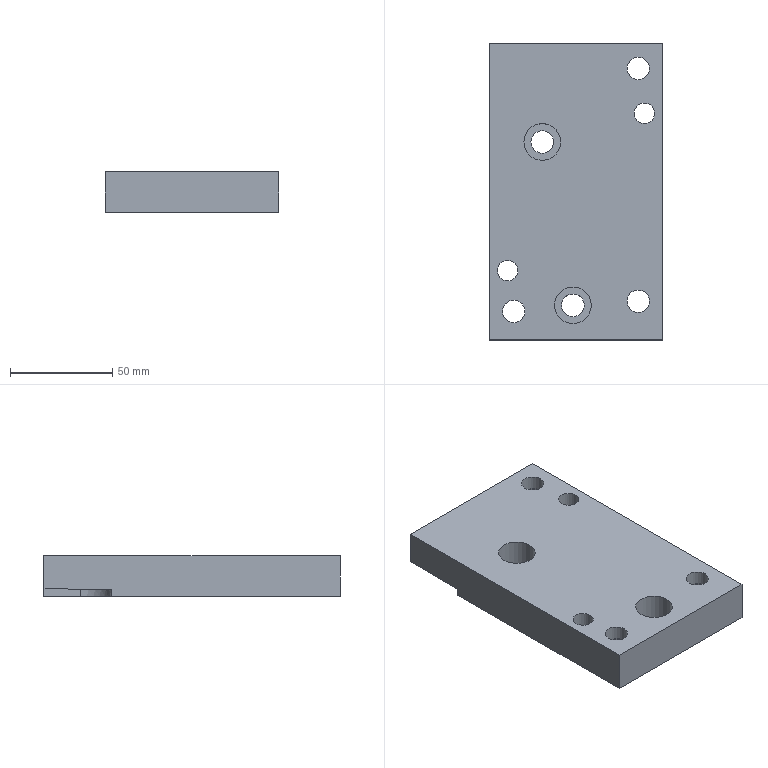Part | STEP file | 404_id26_x_t | 1 solid | 31 faces | box 85 x 145 x 20 mm | volume 217008 mm3 | plane 16 | cylinder 15 | commonest cylinder face diameters 11 x3 17 x3 10 x2 11.1 x2 12 x2 18 x2